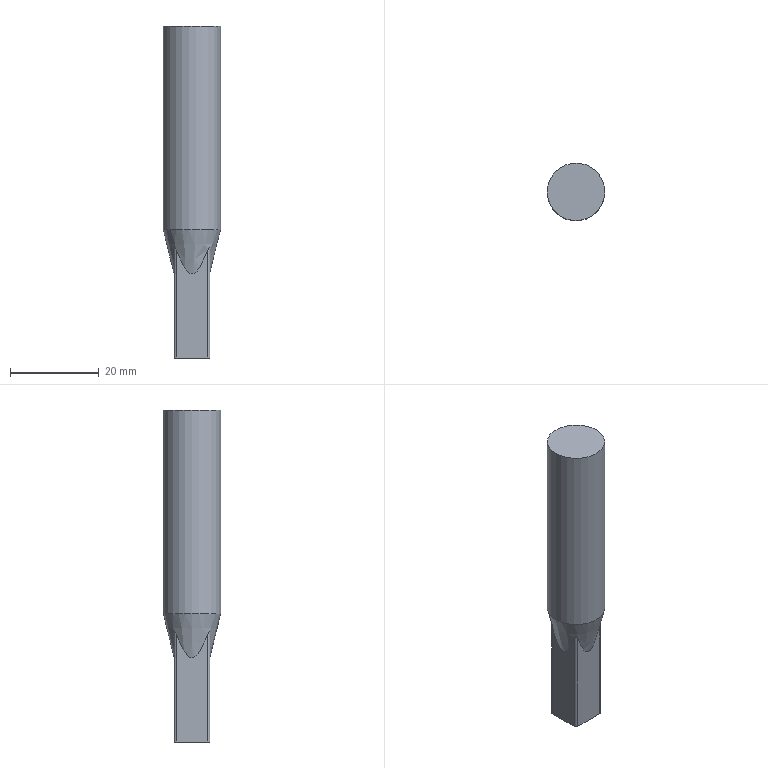Part | NX | features solid 2 | 1 solid | 12 faces | box 13 x 13 x 75 mm | volume 8265 mm3 | plane 6 | cylinder 5 | cone 1 | commonest cylinder face diameters 1.1 x4 13 x1
STEP:
#1=CARTESIAN_POINT('',(330.886,-217.182,47.));
#2=VERTEX_POINT('',#1);
#3=CARTESIAN_POINT('',(323.886,-217.19,47.));
#4=VERTEX_POINT('',#3);
#5=CARTESIAN_POINT('',(327.386,-217.186,47.));
#6=DIRECTION('',(-1.,-0.001244,0.));
#7=VECTOR('',#6,1000.);
#8=LINE('',#5,#7);
#9=EDGE_CURVE('',#2,#4,#8,.T.);
#10=ORIENTED_EDGE('',*,*,#9,.F.);
#11=CARTESIAN_POINT('',(330.886,-217.182,71.318));
#12=VERTEX_POINT('',#11);
#13=CARTESIAN_POINT('',(330.886,-217.182,47.));
#14=DIRECTION('',(0.,0.,1.));
#15=VECTOR('',#14,1000.);
#16=LINE('',#13,#15);
#17=EDGE_CURVE('',#12,#2,#16,.F.);
#18=ORIENTED_EDGE('',*,*,#17,.F.);
#19=CARTESIAN_POINT('',(323.886,-217.19,71.318));
#20=VERTEX_POINT('',#19);
#21=CARTESIAN_POINT('',(330.886,-217.182,71.318));
#22=CARTESIAN_POINT('',(330.693,-217.182,70.802));
#23=CARTESIAN_POINT('',(330.292,-217.183,69.779));
#24=CARTESIAN_POINT('',(329.609,-217.183,68.269));
#25=CARTESIAN_POINT('',(328.926,-217.184,67.081));
#26=CARTESIAN_POINT('',(328.187,-217.185,66.245));
#27=CARTESIAN_POINT('',(327.376,-217.186,65.874));
#28=CARTESIAN_POINT('',(326.569,-217.187,66.259));
#29=CARTESIAN_POINT('',(325.841,-217.188,67.088));
#30=CARTESIAN_POINT('',(325.151,-217.189,68.291));
#31=CARTESIAN_POINT('',(324.478,-217.19,69.784));
#32=CARTESIAN_POINT('',(324.078,-217.19,70.804));
#33=CARTESIAN_POINT('',(323.886,-217.19,71.318));
#34=B_SPLINE_CURVE_WITH_KNOTS('',3,(#21,#22,#23,#24,#25,#26,#27,#28,#29,#30,#31,#32,#33),.UNSPECIFIED.,.F.,.F.,(4,1,1,1,1,1,1,1,1,1,4),(0.001625,0.003275,0.004925,0.006576,0.007401,0.008226,0.009051,0.009876,0.01153,0.01318,0.01483),.UNSPECIFIED.);
#35=EDGE_CURVE('',#12,#20,#34,.T.);
#36=ORIENTED_EDGE('',*,*,#35,.T.);
#37=CARTESIAN_POINT('',(323.886,-217.19,47.));
#38=DIRECTION('',(0.,0.,1.));
#39=VECTOR('',#38,1000.);
#40=LINE('',#37,#39);
#41=EDGE_CURVE('',#4,#20,#40,.T.);
#42=ORIENTED_EDGE('',*,*,#41,.F.);
#43=EDGE_LOOP('',(#10,#18,#36,#42));
#44=FACE_BOUND('',#43,.T.);
#45=CARTESIAN_POINT('',(327.386,-217.186,47.));
#46=DIRECTION('',(0.001244,-1.,0.));
#47=DIRECTION('',(0.,0.,-1.));
#48=AXIS2_PLACEMENT_3D('',#45,#46,#47);
#49=PLANE('',#48);
#50=ADVANCED_FACE('',(#44),#49,.T.);
#51=CARTESIAN_POINT('',(331.426,-209.631,71.318));
#52=VERTEX_POINT('',#51);
#53=CARTESIAN_POINT('',(331.435,-216.631,71.318));
#54=VERTEX_POINT('',#53);
#55=CARTESIAN_POINT('',(331.426,-209.631,71.318));
#56=CARTESIAN_POINT('',(331.426,-209.824,70.802));
#57=CARTESIAN_POINT('',(331.427,-210.225,69.779));
#58=CARTESIAN_POINT('',(331.428,-210.907,68.269));
#59=CARTESIAN_POINT('',(331.429,-211.59,67.081));
#60=CARTESIAN_POINT('',(331.43,-212.329,66.245));
#61=CARTESIAN_POINT('',(331.431,-213.141,65.874));
#62=CARTESIAN_POINT('',(331.432,-213.948,66.259));
#63=CARTESIAN_POINT('',(331.432,-214.676,67.088));
#64=CARTESIAN_POINT('',(331.433,-215.366,68.291));
#65=CARTESIAN_POINT('',(331.434,-216.039,69.784));
#66=CARTESIAN_POINT('',(331.435,-216.439,70.804));
#67=CARTESIAN_POINT('',(331.435,-216.631,71.318));
#68=B_SPLINE_CURVE_WITH_KNOTS('',3,(#55,#56,#57,#58,#59,#60,#61,#62,#63,#64,#65,#66,#67),.UNSPECIFIED.,.F.,.F.,(4,1,1,1,1,1,1,1,1,1,4),(0.001625,0.003275,0.004925,0.006576,0.007401,0.008226,0.009051,0.009876,0.01153,0.01318,0.01483),.UNSPECIFIED.);
#69=EDGE_CURVE('',#52,#54,#68,.T.);
#70=ORIENTED_EDGE('',*,*,#69,.T.);
#71=CARTESIAN_POINT('',(331.435,-216.631,47.));
#72=VERTEX_POINT('',#71);
#73=CARTESIAN_POINT('',(331.435,-216.631,47.));
#74=DIRECTION('',(0.,0.,1.));
#75=VECTOR('',#74,1000.);
#76=LINE('',#73,#75);
#77=EDGE_CURVE('',#72,#54,#76,.T.);
#78=ORIENTED_EDGE('',*,*,#77,.F.);
#79=CARTESIAN_POINT('',(331.426,-209.631,47.));
#80=VERTEX_POINT('',#79);
#81=CARTESIAN_POINT('',(331.431,-213.131,47.));
#82=DIRECTION('',(0.001244,-1.,0.));
#83=VECTOR('',#82,1000.);
#84=LINE('',#81,#83);
#85=EDGE_CURVE('',#80,#72,#84,.T.);
#86=ORIENTED_EDGE('',*,*,#85,.F.);
#87=CARTESIAN_POINT('',(331.426,-209.631,47.));
#88=DIRECTION('',(0.,0.,1.));
#89=VECTOR('',#88,1000.);
#90=LINE('',#87,#89);
#91=EDGE_CURVE('',#52,#80,#90,.F.);
#92=ORIENTED_EDGE('',*,*,#91,.F.);
#93=EDGE_LOOP('',(#70,#78,#86,#92));
#94=FACE_BOUND('',#93,.T.);
#95=CARTESIAN_POINT('',(331.431,-213.131,47.));
#96=DIRECTION('',(1.,0.001244,0.));
#97=DIRECTION('',(0.,0.,1.));
#98=AXIS2_PLACEMENT_3D('',#95,#96,#97);
#99=PLANE('',#98);
#100=ADVANCED_FACE('',(#94),#99,.T.);
#101=CARTESIAN_POINT('',(323.875,-209.09,71.318));
#102=VERTEX_POINT('',#101);
#103=CARTESIAN_POINT('',(330.875,-209.082,71.318));
#104=VERTEX_POINT('',#103);
#105=CARTESIAN_POINT('',(323.875,-209.09,71.318));
#106=CARTESIAN_POINT('',(324.069,-209.09,70.802));
#107=CARTESIAN_POINT('',(324.469,-209.09,69.779));
#108=CARTESIAN_POINT('',(325.152,-209.089,68.269));
#109=CARTESIAN_POINT('',(325.835,-209.088,67.081));
#110=CARTESIAN_POINT('',(326.574,-209.087,66.245));
#111=CARTESIAN_POINT('',(327.385,-209.086,65.874));
#112=CARTESIAN_POINT('',(328.192,-209.085,66.259));
#113=CARTESIAN_POINT('',(328.921,-209.084,67.088));
#114=CARTESIAN_POINT('',(329.61,-209.083,68.291));
#115=CARTESIAN_POINT('',(330.283,-209.083,69.784));
#116=CARTESIAN_POINT('',(330.683,-209.082,70.804));
#117=CARTESIAN_POINT('',(330.875,-209.082,71.318));
#118=B_SPLINE_CURVE_WITH_KNOTS('',3,(#105,#106,#107,#108,#109,#110,#111,#112,#113,#114,#115,#116,#117),.UNSPECIFIED.,.F.,.F.,(4,1,1,1,1,1,1,1,1,1,4),(0.001625,0.003275,0.004925,0.006576,0.007401,0.008226,0.009051,0.009876,0.01153,0.01318,0.01483),.UNSPECIFIED.);
#119=EDGE_CURVE('',#102,#104,#118,.T.);
#120=ORIENTED_EDGE('',*,*,#119,.T.);
#121=CARTESIAN_POINT('',(330.875,-209.082,47.));
#122=VERTEX_POINT('',#121);
#123=CARTESIAN_POINT('',(330.875,-209.082,47.));
#124=DIRECTION('',(0.,0.,1.));
#125=VECTOR('',#124,1000.);
#126=LINE('',#123,#125);
#127=EDGE_CURVE('',#122,#104,#126,.T.);
#128=ORIENTED_EDGE('',*,*,#127,.F.);
#129=CARTESIAN_POINT('',(323.875,-209.09,47.));
#130=VERTEX_POINT('',#129);
#131=CARTESIAN_POINT('',(327.375,-209.086,47.));
#132=DIRECTION('',(1.,0.001244,0.));
#133=VECTOR('',#132,1000.);
#134=LINE('',#131,#133);
#135=EDGE_CURVE('',#130,#122,#134,.T.);
#136=ORIENTED_EDGE('',*,*,#135,.F.);
#137=CARTESIAN_POINT('',(323.875,-209.09,47.));
#138=DIRECTION('',(0.,0.,1.));
#139=VECTOR('',#138,1000.);
#140=LINE('',#137,#139);
#141=EDGE_CURVE('',#102,#130,#140,.F.);
#142=ORIENTED_EDGE('',*,*,#141,.F.);
#143=EDGE_LOOP('',(#120,#128,#136,#142));
#144=FACE_BOUND('',#143,.T.);
#145=CARTESIAN_POINT('',(327.375,-209.086,47.));
#146=DIRECTION('',(-0.001244,1.,0.));
#147=DIRECTION('',(0.,0.,1.));
#148=AXIS2_PLACEMENT_3D('',#145,#146,#147);
#149=PLANE('',#148);
#150=ADVANCED_FACE('',(#144),#149,.T.);
#151=CARTESIAN_POINT('',(323.335,-216.641,47.));
#152=VERTEX_POINT('',#151);
#153=CARTESIAN_POINT('',(323.326,-209.641,47.));
#154=VERTEX_POINT('',#153);
#155=CARTESIAN_POINT('',(323.331,-213.141,47.));
#156=DIRECTION('',(-0.001244,1.,0.));
#157=VECTOR('',#156,1000.);
#158=LINE('',#155,#157);
#159=EDGE_CURVE('',#152,#154,#158,.T.);
#160=ORIENTED_EDGE('',*,*,#159,.T.);
#161=CARTESIAN_POINT('',(323.876,-209.64,47.));
#162=DIRECTION('',(0.,0.,1.));
#163=DIRECTION('',(1.,0.,0.));
#164=AXIS2_PLACEMENT_3D('',#161,#162,#163);
#165=CIRCLE('',#164,0.55);
#166=EDGE_CURVE('',#130,#154,#165,.T.);
#167=ORIENTED_EDGE('',*,*,#166,.F.);
#168=ORIENTED_EDGE('',*,*,#135,.T.);
#169=CARTESIAN_POINT('',(330.876,-209.632,47.));
#170=DIRECTION('',(0.,0.,1.));
#171=DIRECTION('',(1.,0.,0.));
#172=AXIS2_PLACEMENT_3D('',#169,#170,#171);
#173=CIRCLE('',#172,0.55);
#174=EDGE_CURVE('',#80,#122,#173,.T.);
#175=ORIENTED_EDGE('',*,*,#174,.F.);
#176=ORIENTED_EDGE('',*,*,#85,.T.);
#177=CARTESIAN_POINT('',(330.885,-216.632,47.));
#178=DIRECTION('',(0.,0.,1.));
#179=DIRECTION('',(1.,0.,0.));
#180=AXIS2_PLACEMENT_3D('',#177,#178,#179);
#181=CIRCLE('',#180,0.55);
#182=EDGE_CURVE('',#2,#72,#181,.T.);
#183=ORIENTED_EDGE('',*,*,#182,.F.);
#184=ORIENTED_EDGE('',*,*,#9,.T.);
#185=CARTESIAN_POINT('',(323.885,-216.64,47.));
#186=DIRECTION('',(0.,0.,1.));
#187=DIRECTION('',(1.,0.,0.));
#188=AXIS2_PLACEMENT_3D('',#185,#186,#187);
#189=CIRCLE('',#188,0.55);
#190=EDGE_CURVE('',#152,#4,#189,.T.);
#191=ORIENTED_EDGE('',*,*,#190,.F.);
#192=EDGE_LOOP('',(#160,#167,#168,#175,#176,#183,#184,#191));
#193=FACE_BOUND('',#192,.T.);
#194=CARTESIAN_POINT('',(327.381,-213.136,47.));
#195=DIRECTION('',(0.,0.,-1.));
#196=DIRECTION('',(1.,0.001244,0.));
#197=AXIS2_PLACEMENT_3D('',#194,#195,#196);
#198=PLANE('',#197);
#199=ADVANCED_FACE('',(#193),#198,.T.);
#200=CARTESIAN_POINT('',(323.335,-216.641,71.318));
#201=VERTEX_POINT('',#200);
#202=CARTESIAN_POINT('',(323.326,-209.641,71.318));
#203=VERTEX_POINT('',#202);
#204=CARTESIAN_POINT('',(323.335,-216.641,71.318));
#205=CARTESIAN_POINT('',(323.335,-216.448,70.802));
#206=CARTESIAN_POINT('',(323.334,-216.047,69.779));
#207=CARTESIAN_POINT('',(323.333,-215.365,68.269));
#208=CARTESIAN_POINT('',(323.332,-214.682,67.081));
#209=CARTESIAN_POINT('',(323.332,-213.943,66.245));
#210=CARTESIAN_POINT('',(323.331,-213.131,65.874));
#211=CARTESIAN_POINT('',(323.329,-212.324,66.259));
#212=CARTESIAN_POINT('',(323.329,-211.596,67.088));
#213=CARTESIAN_POINT('',(323.328,-210.906,68.291));
#214=CARTESIAN_POINT('',(323.327,-210.234,69.784));
#215=CARTESIAN_POINT('',(323.326,-209.834,70.804));
#216=CARTESIAN_POINT('',(323.326,-209.641,71.318));
#217=B_SPLINE_CURVE_WITH_KNOTS('',3,(#204,#205,#206,#207,#208,#209,#210,#211,#212,#213,#214,#215,#216),.UNSPECIFIED.,.F.,.F.,(4,1,1,1,1,1,1,1,1,1,4),(0.001625,0.003275,0.004925,0.006576,0.007401,0.008226,0.009051,0.009876,0.01153,0.01318,0.01483),.UNSPECIFIED.);
#218=EDGE_CURVE('',#201,#203,#217,.T.);
#219=ORIENTED_EDGE('',*,*,#218,.T.);
#220=CARTESIAN_POINT('',(323.326,-209.641,47.));
#221=DIRECTION('',(0.,0.,1.));
#222=VECTOR('',#221,1000.);
#223=LINE('',#220,#222);
#224=EDGE_CURVE('',#154,#203,#223,.T.);
#225=ORIENTED_EDGE('',*,*,#224,.F.);
#226=ORIENTED_EDGE('',*,*,#159,.F.);
#227=CARTESIAN_POINT('',(323.335,-216.641,47.));
#228=DIRECTION('',(0.,0.,1.));
#229=VECTOR('',#228,1000.);
#230=LINE('',#227,#229);
#231=EDGE_CURVE('',#201,#152,#230,.F.);
#232=ORIENTED_EDGE('',*,*,#231,.F.);
#233=EDGE_LOOP('',(#219,#225,#226,#232));
#234=FACE_BOUND('',#233,.T.);
#235=CARTESIAN_POINT('',(323.331,-213.141,47.));
#236=DIRECTION('',(-1.,-0.001244,0.));
#237=DIRECTION('',(0.,0.,-1.));
#238=AXIS2_PLACEMENT_3D('',#235,#236,#237);
#239=PLANE('',#238);
#240=ADVANCED_FACE('',(#234),#239,.T.);
#241=ORIENTED_EDGE('',*,*,#218,.F.);
#242=CARTESIAN_POINT('',(323.886,-217.19,71.318));
#243=CARTESIAN_POINT('',(323.84,-217.191,71.438));
#244=CARTESIAN_POINT('',(323.758,-217.192,71.659));
#245=CARTESIAN_POINT('',(323.47,-217.053,72.047));
#246=CARTESIAN_POINT('',(323.334,-216.768,71.657));
#247=CARTESIAN_POINT('',(323.335,-216.686,71.438));
#248=CARTESIAN_POINT('',(323.335,-216.641,71.318));
#249=B_SPLINE_CURVE_WITH_KNOTS('',3,(#242,#243,#244,#245,#246,#247,#248),.UNSPECIFIED.,.F.,.F.,(4,1,1,1,4),(0.,0.0003842,0.0007683,0.001152,0.001537),.UNSPECIFIED.);
#250=EDGE_CURVE('',#20,#201,#249,.T.);
#251=ORIENTED_EDGE('',*,*,#250,.F.);
#252=ORIENTED_EDGE('',*,*,#35,.F.);
#253=CARTESIAN_POINT('',(331.435,-216.631,71.318));
#254=CARTESIAN_POINT('',(331.435,-216.676,71.438));
#255=CARTESIAN_POINT('',(331.436,-216.758,71.659));
#256=CARTESIAN_POINT('',(331.298,-217.046,72.047));
#257=CARTESIAN_POINT('',(331.013,-217.182,71.657));
#258=CARTESIAN_POINT('',(330.931,-217.182,71.438));
#259=CARTESIAN_POINT('',(330.886,-217.182,71.318));
#260=B_SPLINE_CURVE_WITH_KNOTS('',3,(#253,#254,#255,#256,#257,#258,#259),.UNSPECIFIED.,.F.,.F.,(4,1,1,1,4),(0.,0.0003842,0.0007683,0.001152,0.001537),.UNSPECIFIED.);
#261=EDGE_CURVE('',#54,#12,#260,.T.);
#262=ORIENTED_EDGE('',*,*,#261,.F.);
#263=ORIENTED_EDGE('',*,*,#69,.F.);
#264=CARTESIAN_POINT('',(330.875,-209.082,71.318));
#265=CARTESIAN_POINT('',(330.921,-209.082,71.438));
#266=CARTESIAN_POINT('',(331.003,-209.08,71.659));
#267=CARTESIAN_POINT('',(331.291,-209.219,72.047));
#268=CARTESIAN_POINT('',(331.427,-209.504,71.657));
#269=CARTESIAN_POINT('',(331.426,-209.586,71.438));
#270=CARTESIAN_POINT('',(331.426,-209.631,71.318));
#271=B_SPLINE_CURVE_WITH_KNOTS('',3,(#264,#265,#266,#267,#268,#269,#270),.UNSPECIFIED.,.F.,.F.,(4,1,1,1,4),(0.,0.0003842,0.0007683,0.001152,0.001537),.UNSPECIFIED.);
#272=EDGE_CURVE('',#104,#52,#271,.T.);
#273=ORIENTED_EDGE('',*,*,#272,.F.);
#274=ORIENTED_EDGE('',*,*,#119,.F.);
#275=CARTESIAN_POINT('',(323.326,-209.641,71.318));
#276=CARTESIAN_POINT('',(323.326,-209.596,71.438));
#277=CARTESIAN_POINT('',(323.325,-209.514,71.659));
#278=CARTESIAN_POINT('',(323.463,-209.226,72.047));
#279=CARTESIAN_POINT('',(323.748,-209.09,71.657));
#280=CARTESIAN_POINT('',(323.83,-209.091,71.438));
#281=CARTESIAN_POINT('',(323.875,-209.09,71.318));
#282=B_SPLINE_CURVE_WITH_KNOTS('',3,(#275,#276,#277,#278,#279,#280,#281),.UNSPECIFIED.,.F.,.F.,(4,1,1,1,4),(0.,0.0003842,0.0007683,0.001152,0.001537),.UNSPECIFIED.);
#283=EDGE_CURVE('',#203,#102,#282,.T.);
#284=ORIENTED_EDGE('',*,*,#283,.F.);
#285=EDGE_LOOP('',(#241,#251,#252,#262,#263,#273,#274,#284));
#286=FACE_BOUND('',#285,.T.);
#287=CARTESIAN_POINT('',(320.881,-213.144,76.));
#288=VERTEX_POINT('',#287);
#289=CARTESIAN_POINT('',(327.381,-213.136,76.));
#290=DIRECTION('',(0.,0.,-1.));
#291=DIRECTION('',(-1.,-0.001244,0.));
#292=AXIS2_PLACEMENT_3D('',#289,#290,#291);
#293=CIRCLE('',#292,6.5);
#294=EDGE_CURVE('',#288,#288,#293,.T.);
#295=ORIENTED_EDGE('',*,*,#294,.T.);
#296=EDGE_LOOP('',(#295));
#297=FACE_BOUND('',#296,.T.);
#298=CARTESIAN_POINT('',(327.381,-213.136,66.));
#299=DIRECTION('',(0.,0.,1.));
#300=DIRECTION('',(-1.,-0.001244,0.));
#301=AXIS2_PLACEMENT_3D('',#298,#299,#300);
#302=CONICAL_SURFACE('',#301,4.05,0.2403);
#303=ADVANCED_FACE('',(#286,#297),#302,.T.);
#304=CARTESIAN_POINT('',(333.881,-213.128,122.));
#305=VERTEX_POINT('',#304);
#306=CARTESIAN_POINT('',(327.381,-213.136,122.));
#307=DIRECTION('',(0.,0.,1.));
#308=DIRECTION('',(1.,0.001244,0.));
#309=AXIS2_PLACEMENT_3D('',#306,#307,#308);
#310=CIRCLE('',#309,6.5);
#311=EDGE_CURVE('',#305,#305,#310,.T.);
#312=ORIENTED_EDGE('',*,*,#311,.T.);
#313=EDGE_LOOP('',(#312));
#314=FACE_BOUND('',#313,.T.);
#315=CARTESIAN_POINT('',(327.381,-213.136,122.));
#316=DIRECTION('',(0.,0.,1.));
#317=DIRECTION('',(-1.,-0.001244,0.));
#318=AXIS2_PLACEMENT_3D('',#315,#316,#317);
#319=PLANE('',#318);
#320=ADVANCED_FACE('',(#314),#319,.T.);
#321=ORIENTED_EDGE('',*,*,#311,.F.);
#322=EDGE_LOOP('',(#321));
#323=FACE_BOUND('',#322,.T.);
#324=ORIENTED_EDGE('',*,*,#294,.F.);
#325=EDGE_LOOP('',(#324));
#326=FACE_BOUND('',#325,.T.);
#327=CARTESIAN_POINT('',(327.381,-213.136,76.));
#328=DIRECTION('',(0.,0.,1.));
#329=DIRECTION('',(-1.,-0.001244,0.));
#330=AXIS2_PLACEMENT_3D('',#327,#328,#329);
#331=CYLINDRICAL_SURFACE('',#330,6.5);
#332=ADVANCED_FACE('',(#323,#326),#331,.T.);
#333=ORIENTED_EDGE('',*,*,#190,.T.);
#334=ORIENTED_EDGE('',*,*,#41,.T.);
#335=ORIENTED_EDGE('',*,*,#250,.T.);
#336=ORIENTED_EDGE('',*,*,#231,.T.);
#337=EDGE_LOOP('',(#333,#334,#335,#336));
#338=FACE_BOUND('',#337,.T.);
#339=CARTESIAN_POINT('',(323.885,-216.64,47.));
#340=DIRECTION('',(0.,0.,1.));
#341=DIRECTION('',(-1.,0.,0.));
#342=AXIS2_PLACEMENT_3D('',#339,#340,#341);
#343=CYLINDRICAL_SURFACE('',#342,0.55);
#344=ADVANCED_FACE('',(#338),#343,.T.);
#345=ORIENTED_EDGE('',*,*,#166,.T.);
#346=ORIENTED_EDGE('',*,*,#224,.T.);
#347=ORIENTED_EDGE('',*,*,#283,.T.);
#348=ORIENTED_EDGE('',*,*,#141,.T.);
#349=EDGE_LOOP('',(#345,#346,#347,#348));
#350=FACE_BOUND('',#349,.T.);
#351=CARTESIAN_POINT('',(323.876,-209.64,47.));
#352=DIRECTION('',(0.,0.,1.));
#353=DIRECTION('',(-1.,0.,0.));
#354=AXIS2_PLACEMENT_3D('',#351,#352,#353);
#355=CYLINDRICAL_SURFACE('',#354,0.55);
#356=ADVANCED_FACE('',(#350),#355,.T.);
#357=ORIENTED_EDGE('',*,*,#174,.T.);
#358=ORIENTED_EDGE('',*,*,#127,.T.);
#359=ORIENTED_EDGE('',*,*,#272,.T.);
#360=ORIENTED_EDGE('',*,*,#91,.T.);
#361=EDGE_LOOP('',(#357,#358,#359,#360));
#362=FACE_BOUND('',#361,.T.);
#363=CARTESIAN_POINT('',(330.876,-209.632,47.));
#364=DIRECTION('',(0.,0.,1.));
#365=DIRECTION('',(-1.,0.,0.));
#366=AXIS2_PLACEMENT_3D('',#363,#364,#365);
#367=CYLINDRICAL_SURFACE('',#366,0.55);
#368=ADVANCED_FACE('',(#362),#367,.T.);
#369=ORIENTED_EDGE('',*,*,#182,.T.);
#370=ORIENTED_EDGE('',*,*,#77,.T.);
#371=ORIENTED_EDGE('',*,*,#261,.T.);
#372=ORIENTED_EDGE('',*,*,#17,.T.);
#373=EDGE_LOOP('',(#369,#370,#371,#372));
#374=FACE_BOUND('',#373,.T.);
#375=CARTESIAN_POINT('',(330.885,-216.632,47.));
#376=DIRECTION('',(0.,0.,1.));
#377=DIRECTION('',(-1.,0.,0.));
#378=AXIS2_PLACEMENT_3D('',#375,#376,#377);
#379=CYLINDRICAL_SURFACE('',#378,0.55);
#380=ADVANCED_FACE('',(#374),#379,.T.);
#381=CLOSED_SHELL('',(#50,#100,#150,#199,#240,#303,#320,#332,#344,#356,#368,#380));
#382=MANIFOLD_SOLID_BREP('',#381);
#383=(LENGTH_UNIT()NAMED_UNIT(*)SI_UNIT(.MILLI.,.METRE.));
#384=UNCERTAINTY_MEASURE_WITH_UNIT(LENGTH_MEASURE(0.0508),#383,'','');
#385=(NAMED_UNIT(*)PLANE_ANGLE_UNIT()SI_UNIT($,.RADIAN.));
#386=(NAMED_UNIT(*)SI_UNIT($,.STERADIAN.)SOLID_ANGLE_UNIT());
#387=(GEOMETRIC_REPRESENTATION_CONTEXT(3)GLOBAL_UNCERTAINTY_ASSIGNED_CONTEXT((#384))GLOBAL_UNIT_ASSIGNED_CONTEXT((#383,#385,#386))REPRESENTATION_CONTEXT('',''));
#388=ADVANCED_BREP_SHAPE_REPRESENTATION('',(#382),#387);